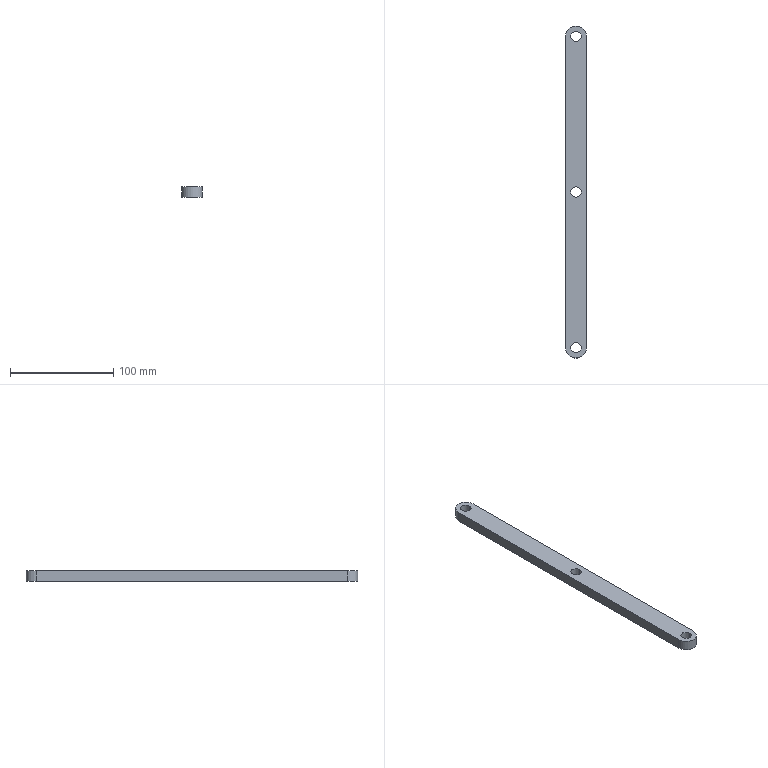Part | SolidWorks | 1 solid | 12 faces | box 20 x 321 x 10 mm | volume 60985 mm3 | cylinder 8 | plane 4 | commonest cylinder face diameters 10 x6 20 x2
STEP:
#1=CARTESIAN_POINT('',(-5.,0.,10.));
#2=VERTEX_POINT('',#1);
#3=CARTESIAN_POINT('',(5.,0.,10.));
#4=VERTEX_POINT('',#3);
#5=CARTESIAN_POINT('',(0.,0.,10.));
#6=DIRECTION('',(0.,0.,1.));
#7=DIRECTION('',(1.,0.,0.));
#8=AXIS2_PLACEMENT_3D('',#5,#6,#7);
#9=CIRCLE('',#8,5.);
#10=EDGE_CURVE('',#2,#4,#9,.T.);
#11=ORIENTED_EDGE('',*,*,#10,.T.);
#12=CARTESIAN_POINT('',(5.,0.,0.));
#13=VERTEX_POINT('',#12);
#14=CARTESIAN_POINT('',(5.,0.,10.));
#15=DIRECTION('',(0.,0.,-1.));
#16=VECTOR('',#15,1000.);
#17=LINE('',#14,#16);
#18=EDGE_CURVE('',#4,#13,#17,.T.);
#19=ORIENTED_EDGE('',*,*,#18,.T.);
#20=CARTESIAN_POINT('',(-5.,0.,0.));
#21=VERTEX_POINT('',#20);
#22=CARTESIAN_POINT('',(0.,0.,0.));
#23=DIRECTION('',(0.,0.,1.));
#24=DIRECTION('',(1.,0.,0.));
#25=AXIS2_PLACEMENT_3D('',#22,#23,#24);
#26=CIRCLE('',#25,5.);
#27=EDGE_CURVE('',#21,#13,#26,.T.);
#28=ORIENTED_EDGE('',*,*,#27,.F.);
#29=CARTESIAN_POINT('',(-5.,0.,10.));
#30=DIRECTION('',(0.,0.,-1.));
#31=VECTOR('',#30,1000.);
#32=LINE('',#29,#31);
#33=EDGE_CURVE('',#2,#21,#32,.T.);
#34=ORIENTED_EDGE('',*,*,#33,.F.);
#35=EDGE_LOOP('',(#11,#19,#28,#34));
#36=FACE_OUTER_BOUND('',#35,.T.);
#37=CARTESIAN_POINT('',(0.,0.,10.));
#38=DIRECTION('',(0.,0.,-1.));
#39=DIRECTION('',(-1.,0.,0.));
#40=AXIS2_PLACEMENT_3D('',#37,#38,#39);
#41=CYLINDRICAL_SURFACE('',#40,5.);
#42=ADVANCED_FACE('',(#36),#41,.F.);
#43=CARTESIAN_POINT('',(-5.,150.5,10.));
#44=VERTEX_POINT('',#43);
#45=CARTESIAN_POINT('',(5.,150.5,10.));
#46=VERTEX_POINT('',#45);
#47=CARTESIAN_POINT('',(0.,150.5,10.));
#48=DIRECTION('',(0.,0.,1.));
#49=DIRECTION('',(1.,0.,0.));
#50=AXIS2_PLACEMENT_3D('',#47,#48,#49);
#51=CIRCLE('',#50,5.);
#52=EDGE_CURVE('',#44,#46,#51,.T.);
#53=ORIENTED_EDGE('',*,*,#52,.T.);
#54=CARTESIAN_POINT('',(5.,150.5,0.));
#55=VERTEX_POINT('',#54);
#56=CARTESIAN_POINT('',(5.,150.5,10.));
#57=DIRECTION('',(0.,0.,-1.));
#58=VECTOR('',#57,1000.);
#59=LINE('',#56,#58);
#60=EDGE_CURVE('',#46,#55,#59,.T.);
#61=ORIENTED_EDGE('',*,*,#60,.T.);
#62=CARTESIAN_POINT('',(-5.,150.5,0.));
#63=VERTEX_POINT('',#62);
#64=CARTESIAN_POINT('',(0.,150.5,0.));
#65=DIRECTION('',(0.,0.,1.));
#66=DIRECTION('',(1.,0.,0.));
#67=AXIS2_PLACEMENT_3D('',#64,#65,#66);
#68=CIRCLE('',#67,5.);
#69=EDGE_CURVE('',#63,#55,#68,.T.);
#70=ORIENTED_EDGE('',*,*,#69,.F.);
#71=CARTESIAN_POINT('',(-5.,150.5,10.));
#72=DIRECTION('',(0.,0.,-1.));
#73=VECTOR('',#72,1000.);
#74=LINE('',#71,#73);
#75=EDGE_CURVE('',#44,#63,#74,.T.);
#76=ORIENTED_EDGE('',*,*,#75,.F.);
#77=EDGE_LOOP('',(#53,#61,#70,#76));
#78=FACE_OUTER_BOUND('',#77,.T.);
#79=CARTESIAN_POINT('',(0.,150.5,10.));
#80=DIRECTION('',(0.,0.,-1.));
#81=DIRECTION('',(-1.,0.,0.));
#82=AXIS2_PLACEMENT_3D('',#79,#80,#81);
#83=CYLINDRICAL_SURFACE('',#82,5.);
#84=ADVANCED_FACE('',(#78),#83,.F.);
#85=CARTESIAN_POINT('',(-5.,301.,10.));
#86=VERTEX_POINT('',#85);
#87=CARTESIAN_POINT('',(5.,301.,10.));
#88=VERTEX_POINT('',#87);
#89=CARTESIAN_POINT('',(0.,301.,10.));
#90=DIRECTION('',(0.,0.,1.));
#91=DIRECTION('',(1.,0.,0.));
#92=AXIS2_PLACEMENT_3D('',#89,#90,#91);
#93=CIRCLE('',#92,5.);
#94=EDGE_CURVE('',#86,#88,#93,.T.);
#95=ORIENTED_EDGE('',*,*,#94,.T.);
#96=CARTESIAN_POINT('',(5.,301.,0.));
#97=VERTEX_POINT('',#96);
#98=CARTESIAN_POINT('',(5.,301.,10.));
#99=DIRECTION('',(0.,0.,-1.));
#100=VECTOR('',#99,1000.);
#101=LINE('',#98,#100);
#102=EDGE_CURVE('',#88,#97,#101,.T.);
#103=ORIENTED_EDGE('',*,*,#102,.T.);
#104=CARTESIAN_POINT('',(-5.,301.,0.));
#105=VERTEX_POINT('',#104);
#106=CARTESIAN_POINT('',(0.,301.,0.));
#107=DIRECTION('',(0.,0.,1.));
#108=DIRECTION('',(1.,0.,0.));
#109=AXIS2_PLACEMENT_3D('',#106,#107,#108);
#110=CIRCLE('',#109,5.);
#111=EDGE_CURVE('',#105,#97,#110,.T.);
#112=ORIENTED_EDGE('',*,*,#111,.F.);
#113=CARTESIAN_POINT('',(-5.,301.,10.));
#114=DIRECTION('',(0.,0.,-1.));
#115=VECTOR('',#114,1000.);
#116=LINE('',#113,#115);
#117=EDGE_CURVE('',#86,#105,#116,.T.);
#118=ORIENTED_EDGE('',*,*,#117,.F.);
#119=EDGE_LOOP('',(#95,#103,#112,#118));
#120=FACE_OUTER_BOUND('',#119,.T.);
#121=CARTESIAN_POINT('',(0.,301.,10.));
#122=DIRECTION('',(0.,0.,-1.));
#123=DIRECTION('',(-1.,0.,0.));
#124=AXIS2_PLACEMENT_3D('',#121,#122,#123);
#125=CYLINDRICAL_SURFACE('',#124,5.);
#126=ADVANCED_FACE('',(#120),#125,.F.);
#127=ORIENTED_EDGE('',*,*,#52,.F.);
#128=CARTESIAN_POINT('',(0.,150.5,10.));
#129=DIRECTION('',(0.,0.,1.));
#130=DIRECTION('',(1.,0.,0.));
#131=AXIS2_PLACEMENT_3D('',#128,#129,#130);
#132=CIRCLE('',#131,5.);
#133=EDGE_CURVE('',#46,#44,#132,.T.);
#134=ORIENTED_EDGE('',*,*,#133,.F.);
#135=EDGE_LOOP('',(#127,#134));
#136=FACE_BOUND('',#135,.T.);
#137=CARTESIAN_POINT('',(-10.,0.,10.));
#138=VERTEX_POINT('',#137);
#139=CARTESIAN_POINT('',(10.,0.,10.));
#140=VERTEX_POINT('',#139);
#141=CARTESIAN_POINT('',(0.,0.,10.));
#142=DIRECTION('',(0.,0.,1.));
#143=DIRECTION('',(1.,0.,0.));
#144=AXIS2_PLACEMENT_3D('',#141,#142,#143);
#145=CIRCLE('',#144,10.);
#146=EDGE_CURVE('',#138,#140,#145,.T.);
#147=ORIENTED_EDGE('',*,*,#146,.T.);
#148=CARTESIAN_POINT('',(10.,301.,10.));
#149=VERTEX_POINT('',#148);
#150=CARTESIAN_POINT('',(10.,0.,10.));
#151=DIRECTION('',(0.,1.,0.));
#152=VECTOR('',#151,1000.);
#153=LINE('',#150,#152);
#154=EDGE_CURVE('',#140,#149,#153,.T.);
#155=ORIENTED_EDGE('',*,*,#154,.T.);
#156=CARTESIAN_POINT('',(-10.,301.,10.));
#157=VERTEX_POINT('',#156);
#158=CARTESIAN_POINT('',(0.,301.,10.));
#159=DIRECTION('',(0.,0.,1.));
#160=DIRECTION('',(1.,0.,0.));
#161=AXIS2_PLACEMENT_3D('',#158,#159,#160);
#162=CIRCLE('',#161,10.);
#163=EDGE_CURVE('',#149,#157,#162,.T.);
#164=ORIENTED_EDGE('',*,*,#163,.T.);
#165=CARTESIAN_POINT('',(-10.,0.,10.));
#166=DIRECTION('',(0.,-1.,0.));
#167=VECTOR('',#166,1000.);
#168=LINE('',#165,#167);
#169=EDGE_CURVE('',#157,#138,#168,.T.);
#170=ORIENTED_EDGE('',*,*,#169,.T.);
#171=EDGE_LOOP('',(#147,#155,#164,#170));
#172=FACE_OUTER_BOUND('',#171,.T.);
#173=ORIENTED_EDGE('',*,*,#94,.F.);
#174=CARTESIAN_POINT('',(0.,301.,10.));
#175=DIRECTION('',(0.,0.,1.));
#176=DIRECTION('',(1.,0.,0.));
#177=AXIS2_PLACEMENT_3D('',#174,#175,#176);
#178=CIRCLE('',#177,5.);
#179=EDGE_CURVE('',#88,#86,#178,.T.);
#180=ORIENTED_EDGE('',*,*,#179,.F.);
#181=EDGE_LOOP('',(#173,#180));
#182=FACE_BOUND('',#181,.T.);
#183=ORIENTED_EDGE('',*,*,#10,.F.);
#184=CARTESIAN_POINT('',(0.,0.,10.));
#185=DIRECTION('',(0.,0.,1.));
#186=DIRECTION('',(1.,0.,0.));
#187=AXIS2_PLACEMENT_3D('',#184,#185,#186);
#188=CIRCLE('',#187,5.);
#189=EDGE_CURVE('',#4,#2,#188,.T.);
#190=ORIENTED_EDGE('',*,*,#189,.F.);
#191=EDGE_LOOP('',(#183,#190));
#192=FACE_BOUND('',#191,.T.);
#193=CARTESIAN_POINT('',(0.,0.,10.));
#194=DIRECTION('',(0.,0.,1.));
#195=DIRECTION('',(1.,0.,0.));
#196=AXIS2_PLACEMENT_3D('',#193,#194,#195);
#197=PLANE('',#196);
#198=ADVANCED_FACE('',(#136,#172,#182,#192),#197,.T.);
#199=CARTESIAN_POINT('',(-10.,0.,0.));
#200=VERTEX_POINT('',#199);
#201=CARTESIAN_POINT('',(10.,0.,0.));
#202=VERTEX_POINT('',#201);
#203=CARTESIAN_POINT('',(0.,0.,0.));
#204=DIRECTION('',(0.,0.,1.));
#205=DIRECTION('',(1.,0.,0.));
#206=AXIS2_PLACEMENT_3D('',#203,#204,#205);
#207=CIRCLE('',#206,10.);
#208=EDGE_CURVE('',#200,#202,#207,.T.);
#209=ORIENTED_EDGE('',*,*,#208,.F.);
#210=CARTESIAN_POINT('',(-10.,301.,0.));
#211=VERTEX_POINT('',#210);
#212=CARTESIAN_POINT('',(-10.,0.,0.));
#213=DIRECTION('',(0.,-1.,0.));
#214=VECTOR('',#213,1000.);
#215=LINE('',#212,#214);
#216=EDGE_CURVE('',#211,#200,#215,.T.);
#217=ORIENTED_EDGE('',*,*,#216,.F.);
#218=CARTESIAN_POINT('',(10.,301.,0.));
#219=VERTEX_POINT('',#218);
#220=CARTESIAN_POINT('',(0.,301.,0.));
#221=DIRECTION('',(0.,0.,1.));
#222=DIRECTION('',(1.,0.,0.));
#223=AXIS2_PLACEMENT_3D('',#220,#221,#222);
#224=CIRCLE('',#223,10.);
#225=EDGE_CURVE('',#219,#211,#224,.T.);
#226=ORIENTED_EDGE('',*,*,#225,.F.);
#227=CARTESIAN_POINT('',(10.,0.,0.));
#228=DIRECTION('',(0.,1.,0.));
#229=VECTOR('',#228,1000.);
#230=LINE('',#227,#229);
#231=EDGE_CURVE('',#202,#219,#230,.T.);
#232=ORIENTED_EDGE('',*,*,#231,.F.);
#233=EDGE_LOOP('',(#209,#217,#226,#232));
#234=FACE_OUTER_BOUND('',#233,.T.);
#235=ORIENTED_EDGE('',*,*,#111,.T.);
#236=CARTESIAN_POINT('',(0.,301.,0.));
#237=DIRECTION('',(0.,0.,1.));
#238=DIRECTION('',(1.,0.,0.));
#239=AXIS2_PLACEMENT_3D('',#236,#237,#238);
#240=CIRCLE('',#239,5.);
#241=EDGE_CURVE('',#97,#105,#240,.T.);
#242=ORIENTED_EDGE('',*,*,#241,.T.);
#243=EDGE_LOOP('',(#235,#242));
#244=FACE_BOUND('',#243,.T.);
#245=ORIENTED_EDGE('',*,*,#69,.T.);
#246=CARTESIAN_POINT('',(0.,150.5,0.));
#247=DIRECTION('',(0.,0.,1.));
#248=DIRECTION('',(1.,0.,0.));
#249=AXIS2_PLACEMENT_3D('',#246,#247,#248);
#250=CIRCLE('',#249,5.);
#251=EDGE_CURVE('',#55,#63,#250,.T.);
#252=ORIENTED_EDGE('',*,*,#251,.T.);
#253=EDGE_LOOP('',(#245,#252));
#254=FACE_BOUND('',#253,.T.);
#255=ORIENTED_EDGE('',*,*,#27,.T.);
#256=CARTESIAN_POINT('',(0.,0.,0.));
#257=DIRECTION('',(0.,0.,1.));
#258=DIRECTION('',(1.,0.,0.));
#259=AXIS2_PLACEMENT_3D('',#256,#257,#258);
#260=CIRCLE('',#259,5.);
#261=EDGE_CURVE('',#13,#21,#260,.T.);
#262=ORIENTED_EDGE('',*,*,#261,.T.);
#263=EDGE_LOOP('',(#255,#262));
#264=FACE_BOUND('',#263,.T.);
#265=CARTESIAN_POINT('',(0.,0.,0.));
#266=DIRECTION('',(0.,0.,1.));
#267=DIRECTION('',(1.,0.,0.));
#268=AXIS2_PLACEMENT_3D('',#265,#266,#267);
#269=PLANE('',#268);
#270=ADVANCED_FACE('',(#234,#244,#254,#264),#269,.F.);
#271=ORIENTED_EDGE('',*,*,#208,.T.);
#272=CARTESIAN_POINT('',(10.,0.,10.));
#273=DIRECTION('',(0.,0.,-1.));
#274=VECTOR('',#273,1000.);
#275=LINE('',#272,#274);
#276=EDGE_CURVE('',#140,#202,#275,.T.);
#277=ORIENTED_EDGE('',*,*,#276,.F.);
#278=ORIENTED_EDGE('',*,*,#146,.F.);
#279=CARTESIAN_POINT('',(-10.,0.,10.));
#280=DIRECTION('',(0.,0.,-1.));
#281=VECTOR('',#280,1000.);
#282=LINE('',#279,#281);
#283=EDGE_CURVE('',#138,#200,#282,.T.);
#284=ORIENTED_EDGE('',*,*,#283,.T.);
#285=EDGE_LOOP('',(#271,#277,#278,#284));
#286=FACE_OUTER_BOUND('',#285,.T.);
#287=CARTESIAN_POINT('',(0.,0.,10.));
#288=DIRECTION('',(0.,0.,-1.));
#289=DIRECTION('',(-1.,0.,0.));
#290=AXIS2_PLACEMENT_3D('',#287,#288,#289);
#291=CYLINDRICAL_SURFACE('',#290,10.);
#292=ADVANCED_FACE('',(#286),#291,.T.);
#293=ORIENTED_EDGE('',*,*,#231,.T.);
#294=CARTESIAN_POINT('',(10.,301.,10.));
#295=DIRECTION('',(0.,0.,-1.));
#296=VECTOR('',#295,1000.);
#297=LINE('',#294,#296);
#298=EDGE_CURVE('',#149,#219,#297,.T.);
#299=ORIENTED_EDGE('',*,*,#298,.F.);
#300=ORIENTED_EDGE('',*,*,#154,.F.);
#301=ORIENTED_EDGE('',*,*,#276,.T.);
#302=EDGE_LOOP('',(#293,#299,#300,#301));
#303=FACE_OUTER_BOUND('',#302,.T.);
#304=CARTESIAN_POINT('',(10.,0.,10.));
#305=DIRECTION('',(-1.,0.,0.));
#306=DIRECTION('',(0.,0.,1.));
#307=AXIS2_PLACEMENT_3D('',#304,#305,#306);
#308=PLANE('',#307);
#309=ADVANCED_FACE('',(#303),#308,.F.);
#310=ORIENTED_EDGE('',*,*,#225,.T.);
#311=CARTESIAN_POINT('',(-10.,301.,10.));
#312=DIRECTION('',(0.,0.,-1.));
#313=VECTOR('',#312,1000.);
#314=LINE('',#311,#313);
#315=EDGE_CURVE('',#157,#211,#314,.T.);
#316=ORIENTED_EDGE('',*,*,#315,.F.);
#317=ORIENTED_EDGE('',*,*,#163,.F.);
#318=ORIENTED_EDGE('',*,*,#298,.T.);
#319=EDGE_LOOP('',(#310,#316,#317,#318));
#320=FACE_OUTER_BOUND('',#319,.T.);
#321=CARTESIAN_POINT('',(0.,301.,10.));
#322=DIRECTION('',(0.,0.,-1.));
#323=DIRECTION('',(-1.,0.,0.));
#324=AXIS2_PLACEMENT_3D('',#321,#322,#323);
#325=CYLINDRICAL_SURFACE('',#324,10.);
#326=ADVANCED_FACE('',(#320),#325,.T.);
#327=ORIENTED_EDGE('',*,*,#216,.T.);
#328=ORIENTED_EDGE('',*,*,#283,.F.);
#329=ORIENTED_EDGE('',*,*,#169,.F.);
#330=ORIENTED_EDGE('',*,*,#315,.T.);
#331=EDGE_LOOP('',(#327,#328,#329,#330));
#332=FACE_OUTER_BOUND('',#331,.T.);
#333=CARTESIAN_POINT('',(-10.,0.,10.));
#334=DIRECTION('',(1.,0.,0.));
#335=DIRECTION('',(0.,0.,-1.));
#336=AXIS2_PLACEMENT_3D('',#333,#334,#335);
#337=PLANE('',#336);
#338=ADVANCED_FACE('',(#332),#337,.F.);
#339=ORIENTED_EDGE('',*,*,#102,.F.);
#340=ORIENTED_EDGE('',*,*,#179,.T.);
#341=ORIENTED_EDGE('',*,*,#117,.T.);
#342=ORIENTED_EDGE('',*,*,#241,.F.);
#343=EDGE_LOOP('',(#339,#340,#341,#342));
#344=FACE_OUTER_BOUND('',#343,.T.);
#345=CARTESIAN_POINT('',(0.,301.,10.));
#346=DIRECTION('',(0.,0.,-1.));
#347=DIRECTION('',(-1.,0.,0.));
#348=AXIS2_PLACEMENT_3D('',#345,#346,#347);
#349=CYLINDRICAL_SURFACE('',#348,5.);
#350=ADVANCED_FACE('',(#344),#349,.F.);
#351=ORIENTED_EDGE('',*,*,#60,.F.);
#352=ORIENTED_EDGE('',*,*,#133,.T.);
#353=ORIENTED_EDGE('',*,*,#75,.T.);
#354=ORIENTED_EDGE('',*,*,#251,.F.);
#355=EDGE_LOOP('',(#351,#352,#353,#354));
#356=FACE_OUTER_BOUND('',#355,.T.);
#357=CARTESIAN_POINT('',(0.,150.5,10.));
#358=DIRECTION('',(0.,0.,-1.));
#359=DIRECTION('',(-1.,0.,0.));
#360=AXIS2_PLACEMENT_3D('',#357,#358,#359);
#361=CYLINDRICAL_SURFACE('',#360,5.);
#362=ADVANCED_FACE('',(#356),#361,.F.);
#363=ORIENTED_EDGE('',*,*,#18,.F.);
#364=ORIENTED_EDGE('',*,*,#189,.T.);
#365=ORIENTED_EDGE('',*,*,#33,.T.);
#366=ORIENTED_EDGE('',*,*,#261,.F.);
#367=EDGE_LOOP('',(#363,#364,#365,#366));
#368=FACE_OUTER_BOUND('',#367,.T.);
#369=CARTESIAN_POINT('',(0.,0.,10.));
#370=DIRECTION('',(0.,0.,-1.));
#371=DIRECTION('',(-1.,0.,0.));
#372=AXIS2_PLACEMENT_3D('',#369,#370,#371);
#373=CYLINDRICAL_SURFACE('',#372,5.);
#374=ADVANCED_FACE('',(#368),#373,.F.);
#375=CLOSED_SHELL('',(#42,#84,#126,#198,#270,#292,#309,#326,#338,#350,#362,#374));
#376=MANIFOLD_SOLID_BREP('',#375);
#377=CARTESIAN_POINT('',(0.,0.,0.));
#378=DIRECTION('',(0.,0.,1.));
#379=DIRECTION('',(1.,0.,0.));
#380=AXIS2_PLACEMENT_3D('',#377,#378,#379);
#381=(LENGTH_UNIT()NAMED_UNIT(*)SI_UNIT(.MILLI.,.METRE.));
#382=UNCERTAINTY_MEASURE_WITH_UNIT(LENGTH_MEASURE(0.00001),#381,'','');
#383=(NAMED_UNIT(*)PLANE_ANGLE_UNIT()SI_UNIT($,.RADIAN.));
#384=(NAMED_UNIT(*)SI_UNIT($,.STERADIAN.)SOLID_ANGLE_UNIT());
#385=(GEOMETRIC_REPRESENTATION_CONTEXT(3)GLOBAL_UNCERTAINTY_ASSIGNED_CONTEXT((#382))GLOBAL_UNIT_ASSIGNED_CONTEXT((#381,#383,#384))REPRESENTATION_CONTEXT('',''));
#386=ADVANCED_BREP_SHAPE_REPRESENTATION('',(#376,#380),#385);